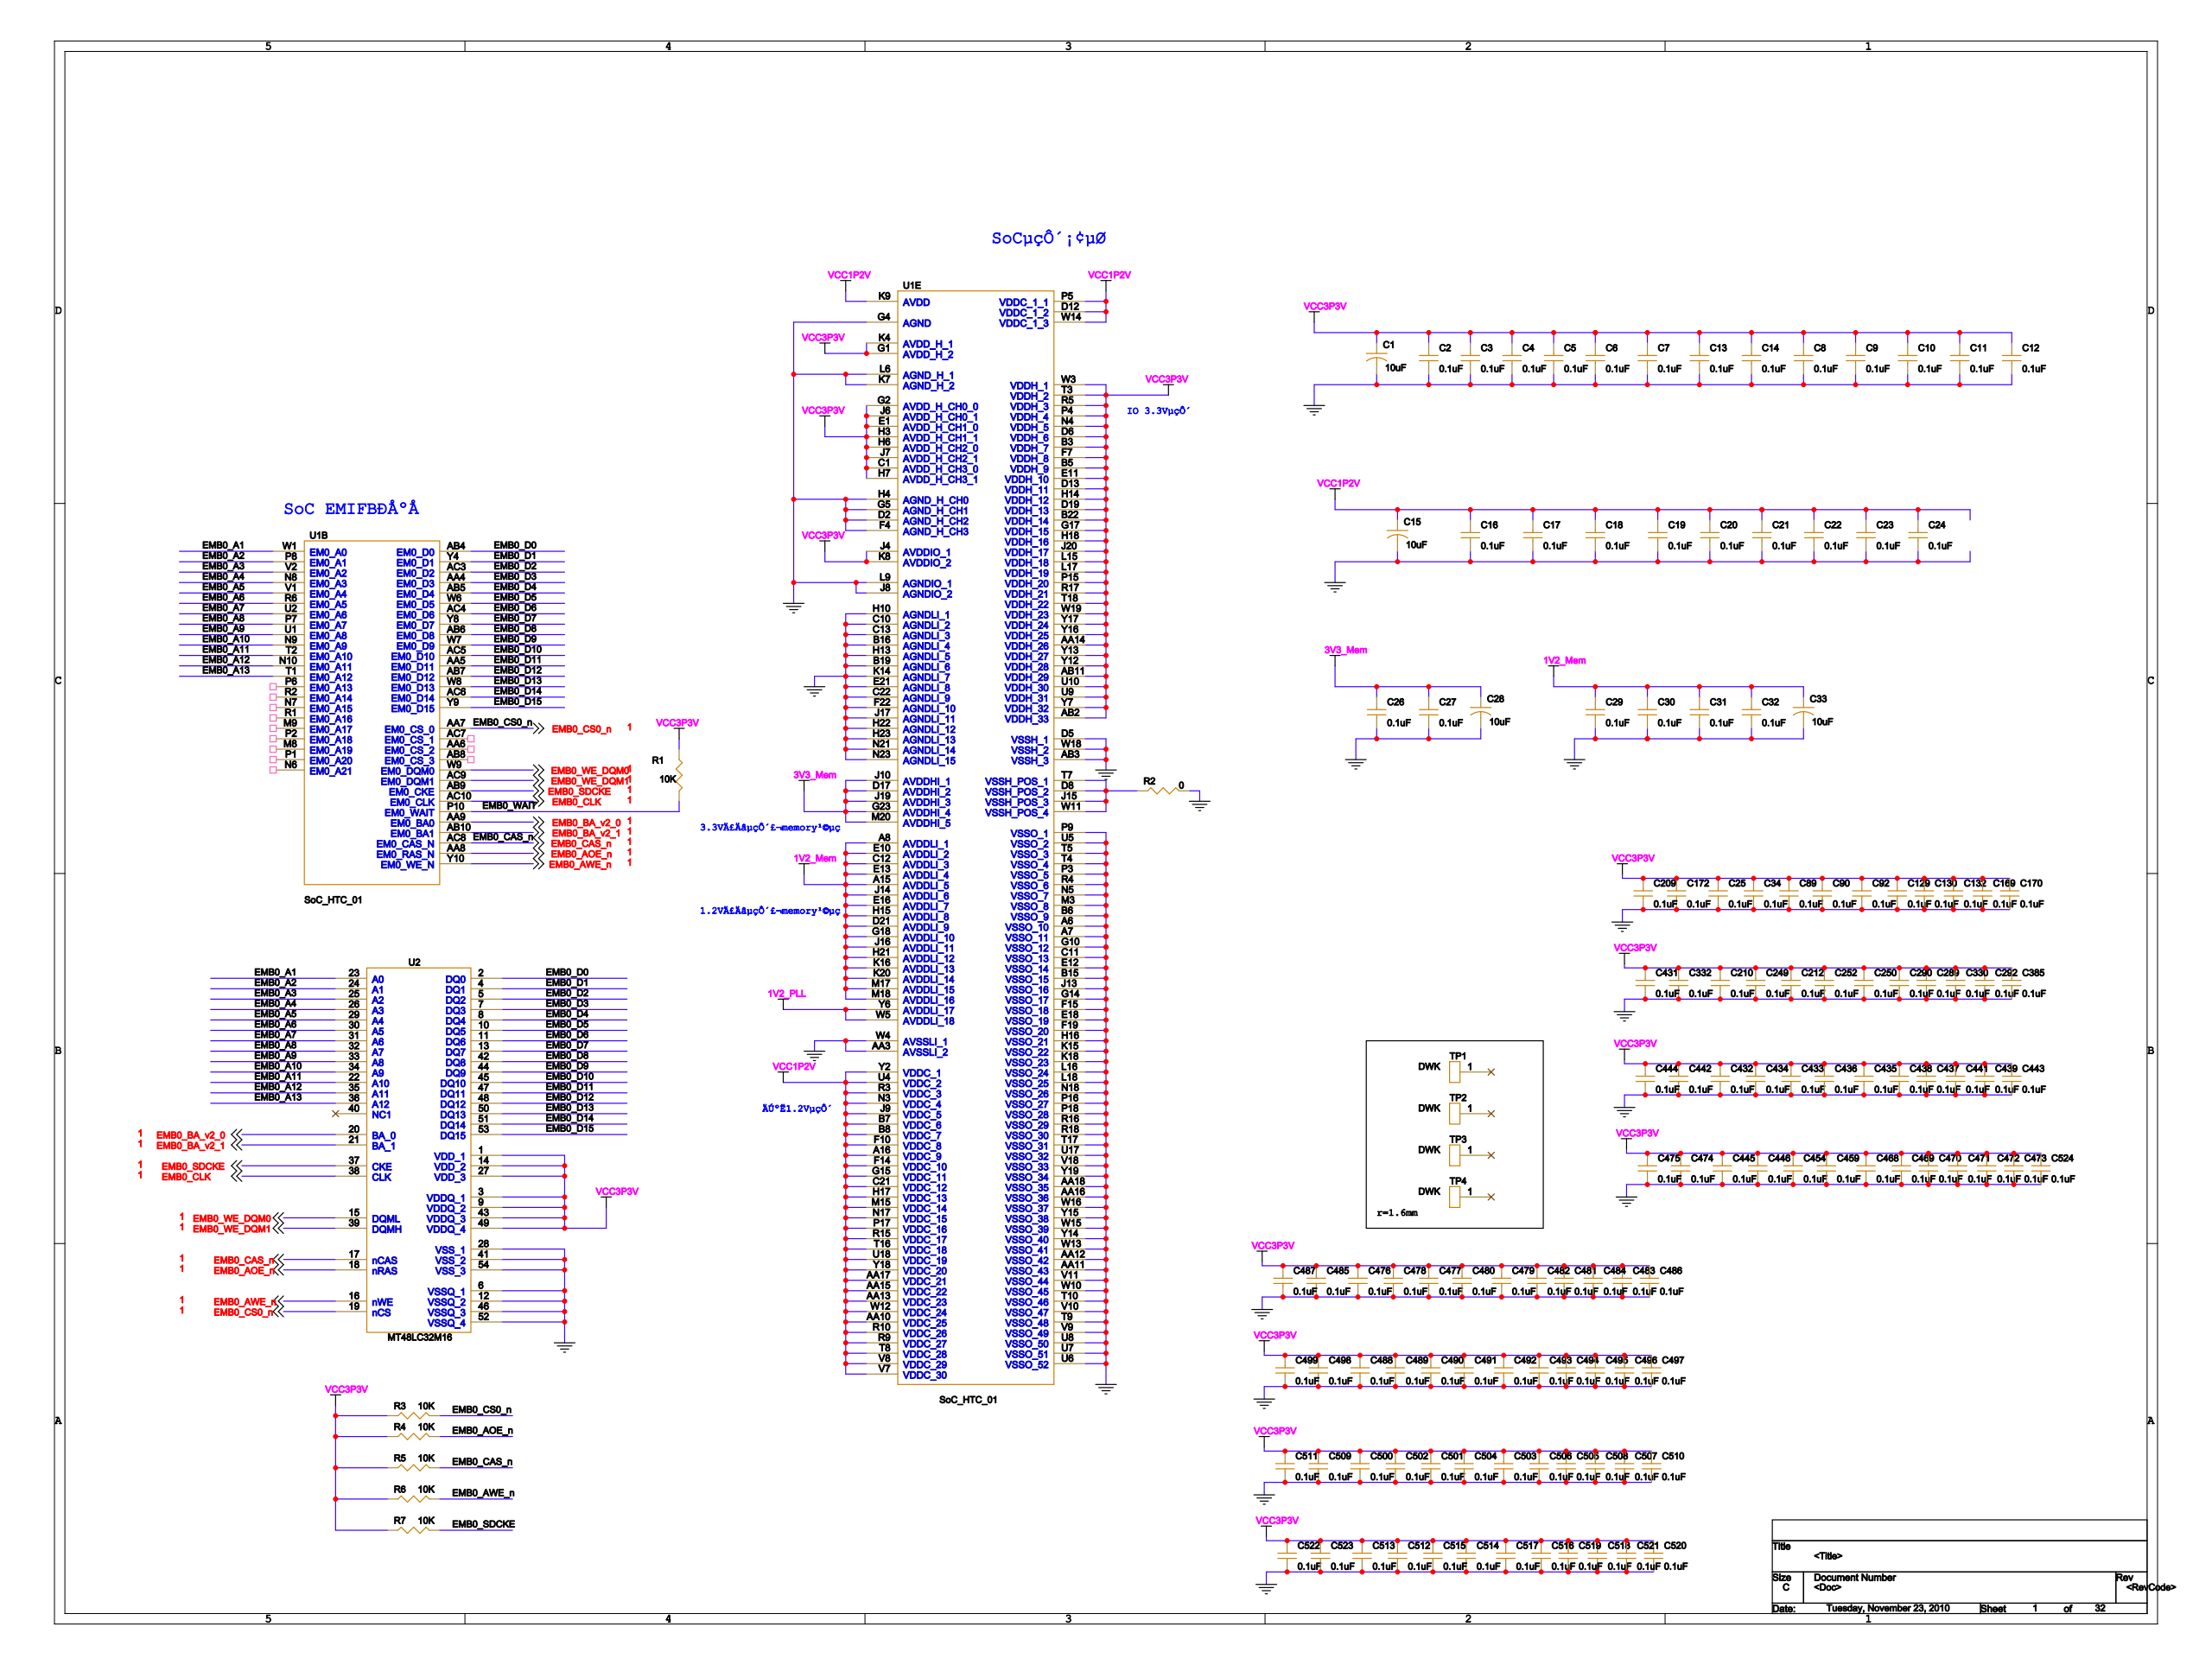Circuit board | Cadence Allegro | 1001 parts | 1318 nets | one sheet of the schematic
Parts on this sheet (reference | value | footprint):
C15 | 10uF | C3216
C25 | 0.1uF | C0402
C28 | 10uF | C3216
C30 | 0.1uF | C0402
C33 | 10uF | C3216
C34 | 0.1uF | C0402
C89 | 0.1uF | C0402
C90 | 0.1uF | C0402
C92 | 0.1uF | C0402
C129 | 0.1uF | C0402
C130 | 0.1uF | C0402
C132 | 0.1uF | C0402
C169 | 0.1uF | C0402
C170 | 0.1uF | C0402
C172 | 0.1uF | C0402
C209 | 0.1uF | C0402
C210 | 0.1uF | C0402
C212 | 0.1uF | C0402
C249 | 0.1uF | C0402
C250 | 0.1uF | C0402
C252 | 0.1uF | C0402
C289 | 0.1uF | C0402
C290 | 0.1uF | C0402
C292 | 0.1uF | C0402
C330 | 0.1uF | C0402
C332 | 0.1uF | C0402
C385 | 0.1uF | C0402
C431 | 0.1uF | C0402
C432 | 0.1uF | C0402
C433 | 0.1uF | C0402
C434 | 0.1uF | C0402
C435 | 0.1uF | C0402
C436 | 0.1uF | C0402
C437 | 0.1uF | C0402
C438 | 0.1uF | C0402
C439 | 0.1uF | C0402
C441 | 0.1uF | C0402
C442 | 0.1uF | C0402
C443 | 0.1uF | C0402
C444 | 0.1uF | C0402
C445 | 0.1uF | C0402
C446 | 0.1uF | C0402
C454 | 0.1uF | C0402
C459 | 0.1uF | C0402
C468 | 0.1uF | C0402
C469 | 0.1uF | C0402
C470 | 0.1uF | C0402
C471 | 0.1uF | C0402
C472 | 0.1uF | C0402
C473 | 0.1uF | C0402
C474 | 0.1uF | C0402
C475 | 0.1uF | C0402
C476 | 0.1uF | C0402
C477 | 0.1uF | C0402
C478 | 0.1uF | C0402
C479 | 0.1uF | C0402
C480 | 0.1uF | C0402
C481 | 0.1uF | C0402
C482 | 0.1uF | C0402
C483 | 0.1uF | C0402
C484 | 0.1uF | C0402
C485 | 0.1uF | C0402
C486 | 0.1uF | C0402
C487 | 0.1uF | C0402
C488 | 0.1uF | C0402
C489 | 0.1uF | C0402
C490 | 0.1uF | C0402
C491 | 0.1uF | C0402
C492 | 0.1uF | C0402
C493 | 0.1uF | C0402
C494 | 0.1uF | C0402
C495 | 0.1uF | C0402
C496 | 0.1uF | C0402
C497 | 0.1uF | C0402
C498 | 0.1uF | C0402
C499 | 0.1uF | C0402
C500 | 0.1uF | C0402
C501 | 0.1uF | C0402
C502 | 0.1uF | C0402
C503 | 0.1uF | C0402
C504 | 0.1uF | C0402
C505 | 0.1uF | C0402
C506 | 0.1uF | C0402
C507 | 0.1uF | C0402
C508 | 0.1uF | C0402
C509 | 0.1uF | C0402
C510 | 0.1uF | C0402
C511 | 0.1uF | C0402
C512 | 0.1uF | C0402
C513 | 0.1uF | C0402
C514 | 0.1uF | C0402
C515 | 0.1uF | C0402
C516 | 0.1uF | C0402
C517 | 0.1uF | C0402
C518 | 0.1uF | C0402
C519 | 0.1uF | C0402
C520 | 0.1uF | C0402
C521 | 0.1uF | C0402
C522 | 0.1uF | C0402
C523 | 0.1uF | C0402
C524 | 0.1uF | C0402
R1 | 10K | 0603
R7 | 10K | 0603
U1 | SoC_HTC_01 | L529_XIN
U2 | MT48LC32M16 | TSOP54
U4 | MAX3243 | TSSOP-28
U6 | MT48LC16M16 | TSOP54
U7 | MT48LC16M16 | TSOP54
U8 | DP83848C | DP83848C_48LQFP
U10 | SoC_HTC_01 | L529_XIN
U17 | MT48LC32M16 | TSOP54
Nets of these parts (net: part-pin ...):
GND: C15-2 C25-2 C28-2 C30-2 C33-2 C34-2 C89-2 C90-2 C92-2 C129-2 C130-2 C132-2 C169-2 C170-2 C172-2 C209-2 C210-2 C212-2 C249-2 C250-2 C252-2 C289-2 C290-2 C292-2 C330-2 C332-2 C385-2 C431-2 C432-2 C433-2 C434-2 C435-2 C436-2 C437-2 C438-2 C439-2 C441-2 C442-2 C443-2 C444-2 C445-2 C446-2 C454-2 C459-2 C468-2 C469-2 C470-2 C471-2 C472-2 C473-2 C474-2 C475-2 C476-2 C477-2 C478-2 C479-2 C480-2 C481-2 C482-2 C483-2 C484-2 C485-2 C486-2 C487-2 C488-2 C489-2 C490-2 C491-2 C492-2 C493-2 C494-2 C495-2 C496-2 C497-2 C498-2 C499-2 C500-2 C501-2 C502-2 C503-2 C504-2 C505-2 C506-2 C507-2 C508-2 C509-2 C510-2 C511-2 C512-2 C513-2 C514-2 C515-2 C516-2 C517-2 C518-2 C519-2 C520-2 C521-2 C522-2 C523-2 C524-2 U1-A6 U1-A7 U1-AA3 U1-AA11 U1-AA12 U1-AA16 U1-AA18 U1-AB3 U1-B6 U1-B15 U1-B16 U1-B19 U1-C10 U1-C11 U1-C13 U1-C22 U1-D2 U1-D5 U1-E12 U1-E18 U1-E21 U1-F4 U1-F15 U1-F19 U1-F22 U1-G4 U1-G5 U1-G10 U1-G14 U1-H4 U1-H10 U1-H13 U1-H16 U1-H22 U1-H23 U1-J8 U1-J13 U1-J17 U1-K7 U1-K14 U1-K15 U1-K18 U1-L6 U1-L9 U1-L16 U1-L18 U1-M3 U1-N5 U1-N18 U1-N21 U1-N23 U1-P3 U1-P9 U1-P16 U1-P18 U1-R4 U1-R16 U1-R18 U1-T4 U1-T5 U1-T9 U1-T10 U1-T17 U1-U5 U1-U6 U1-U7 U1-U8 U1-U17 U1-V9 U1-V10 U1-V11 U1-V18 U1-W4 U1-W10 U1-W13 U1-W15 U1-W16 U1-W18 U1-Y14 U1-Y15 U1-Y19 U2-6 U2-12 U2-28 U2-41 U2-46 U2-52 U2-54 U4-23 U4-25 U6-6 U6-12 U6-28 U6-41 U6-46 U6-52 U6-54 U7-6 U7-12 U7-28 U7-41 U7-46 U7-52 U7-54 U8-15 U8-19 U8-35 U8-36 U8-47 U10-A6 U10-A7 U10-AA3 U10-AA11 U10-AA12 U10-AA16 U10-AA18 U10-AB3 U10-B6 U10-B15 U10-B16 U10-B19 U10-C10 U10-C11 U10-C13 U10-C22 U10-D2 U10-D5 U10-E12 U10-E18 U10-E21 U10-F4 U10-F15 U10-F19 U10-F22 U10-G4 U10-G5 U10-G10 U10-G14 U10-H4 U10-H10 U10-H13 U10-H16 U10-H22 U10-H23 U10-J8 U10-J13 U10-J17 U10-K7 U10-K14 U10-K15 U10-K18 U10-L6 U10-L9 U10-L16 U10-L18 U10-M3 U10-N5 U10-N18 U10-N21 U10-N23 U10-P3 U10-P9 U10-P16 U10-P18 U10-R4 U10-R16 U10-R18 U10-T4 U10-T5 U10-T9 U10-T10 U10-T17 U10-U5 U10-U6 U10-U7 U10-U8 U10-U17 U10-V9 U10-V10 U10-V11 U10-V18 U10-W4 U10-W10 U10-W13 U10-W15 U10-W16 U10-W18 U10-Y14 U10-Y15 U10-Y19 U17-6 U17-12 U17-28 U17-41 U17-46 U17-52 U17-54
VCC3P3V: C25-1 C34-1 C89-1 C90-1 C92-1 C129-1 C130-1 C132-1 C169-1 C170-1 C172-1 C209-1 C210-1 C212-1 C249-1 C250-1 C252-1 C289-1 C290-1 C292-1 C330-1 C332-1 C385-1 C431-1 C432-1 C433-1 C434-1 C435-1 C436-1 C437-1 C438-1 C439-1 C441-1 C442-1 C443-1 C444-1 C445-1 C446-1 C454-1 C459-1 C468-1 C469-1 C470-1 C471-1 C472-1 C473-1 C474-1 C475-1 C476-1 C477-1 C478-1 C479-1 C480-1 C481-1 C482-1 C483-1 C484-1 C485-1 C486-1 C487-1 C488-1 C489-1 C490-1 C491-1 C492-1 C493-1 C494-1 C495-1 C496-1 C497-1 C498-1 C499-1 C500-1 C501-1 C502-1 C503-1 C504-1 C505-1 C506-1 C507-1 C508-1 C509-1 C510-1 C511-1 C512-1 C513-1 C514-1 C515-1 C516-1 C517-1 C518-1 C519-1 C520-1 C521-1 C522-1 C523-1 C524-1 R1-2 R7-1 U1-AA14 U1-AB2 U1-AB11 U1-B3 U1-B5 U1-B22 U1-C1 U1-D6 U1-D13 U1-D19 U1-E1 U1-E11 U1-F7 U1-G1 U1-G2 U1-G17 U1-H3 U1-H6 U1-H7 U1-H14 U1-H18 U1-J4 U1-J6 U1-J7 U1-J20 U1-K4 U1-K8 U1-L15 U1-L17 U1-N4 U1-P4 U1-P15 U1-R5 U1-R17 U1-T3 U1-T18 U1-U9 U1-U10 U1-W3 U1-W19 U1-Y7 U1-Y12 U1-Y13 U1-Y16 U1-Y17 U2-1 U2-3 U2-9 U2-14 U2-27 U2-43 U2-49 U4-22 U4-26 U6-1 U6-3 U6-9 U6-14 U6-27 U6-43 U6-49 U7-1 U7-3 U7-9 U7-14 U7-27 U7-43 U7-49 U8-22 U8-32 U8-48 U10-AA14 U10-AB2 U10-AB11 U10-B3 U10-B5 U10-B22 U10-C1 U10-D6 U10-D13 U10-D19 U10-E1 U10-E11 U10-F7 U10-G1 U10-G2 U10-G17 U10-H3 U10-H6 U10-H7 U10-H14 U10-H18 U10-J4 U10-J6 U10-J7 U10-J20 U10-K4 U10-K8 U10-L15 U10-L17 U10-N4 U10-P4 U10-P15 U10-R5 U10-R17 U10-T3 U10-T18 U10-U9 U10-U10 U10-W3 U10-W19 U10-Y7 U10-Y12 U10-Y13 U10-Y16 U10-Y17 U17-1 U17-3 U17-9 U17-14 U17-27 U17-43 U17-49
VCC1P2V: C15-1 U1-A16 U1-AA10 U1-AA13 U1-AA15 U1-AA17 U1-B7 U1-B8 U1-C21 U1-D12 U1-F10 U1-F14 U1-G15 U1-H17 U1-J9 U1-K9 U1-M15 U1-N3 U1-N17 U1-P5 U1-P17 U1-R3 U1-R9 U1-R10 U1-R15 U1-T8 U1-T16 U1-U4 U1-U18 U1-V7 U1-V8 U1-W12 U1-W14 U1-Y2 U1-Y18 U10-A16 U10-AA10 U10-AA13 U10-AA15 U10-AA17 U10-B7 U10-B8 U10-C21 U10-D12 U10-F10 U10-F14 U10-G15 U10-H17 U10-J9 U10-K9 U10-M15 U10-N3 U10-N17 U10-P5 U10-P17 U10-R3 U10-R9 U10-R10 U10-R15 U10-T8 U10-T16 U10-U4 U10-U18 U10-V7 U10-V8 U10-W12 U10-W14 U10-Y2 U10-Y18
3V3_MEM: C28-1 U1-D17 U1-G23 U1-J10 U1-J19 U1-M20 U10-D17 U10-G23 U10-J10 U10-J19 U10-M20
1V2_MEM: C30-1 C33-1 U1-A8 U1-A15 U1-C12 U1-D21 U1-E10 U1-E13 U1-E16 U1-G18 U1-H15 U1-H21 U1-J14 U1-J16 U1-K16 U1-K20 U1-M17 U1-M18 U10-A8 U10-A15 U10-C12 U10-D21 U10-E10 U10-E13 U10-E16 U10-G18 U10-H15 U10-H21 U10-J14 U10-J16 U10-K16 U10-K20 U10-M17 U10-M18
EMB0_A1: U1-W1 U2-23
EMB0_A2: U1-P8 U2-24
EMB0_A11: U1-T2 U2-22
EMB0_A12: U1-N10 U2-35
EMB0_A13: U1-T1 U2-36
EMB0_A3: U1-V2 U2-25
EMB0_A4: U1-N8 U2-26
EMB0_A5: U1-V1 U2-29
EMB0_A6: U1-R6 U2-30
EMB0_A7: U1-U2 U2-31
EMB0_A8: U1-P7 U2-32
EMB0_A9: U1-U1 U2-33
EMB0_A10: U1-N9 U2-34
EMB0_SDCKE: R7-2 U1-AB9 U2-37
EMB0_CLK: U1-AC10 U2-38
EMB0_D0: U1-AB4 U2-2
EMB0_D1: U1-Y4 U2-4
EMB0_D10: U1-AC5 U2-45
EMB0_D11: U1-AA5 U2-47
EMB0_D12: U1-AB7 U2-48
EMB0_D13: U1-W8 U2-50
EMB0_D14: U1-AC6 U2-51
EMB0_D15: U1-Y9 U2-53
EMB0_D2: U1-AC3 U2-5
EMB0_D3: U1-AA4 U2-7
EMB0_D4: U1-AB5 U2-8
EMB0_D5: U1-W6 U2-10
EMB0_D6: U1-AC4 U2-11
EMB0_D7: U1-Y8 U2-13
EMB0_D8: U1-AB6 U2-42
EMB0_D9: U1-W7 U2-44
EMB0_WE_DQM0: U1-W9 U2-15
EMB0_WE_DQM1: U1-AC9 U2-39
EMB0_WAIT: R1-1 U1-P10
1V2_PLL: U1-W5 U1-Y6 U10-W5 U10-Y6